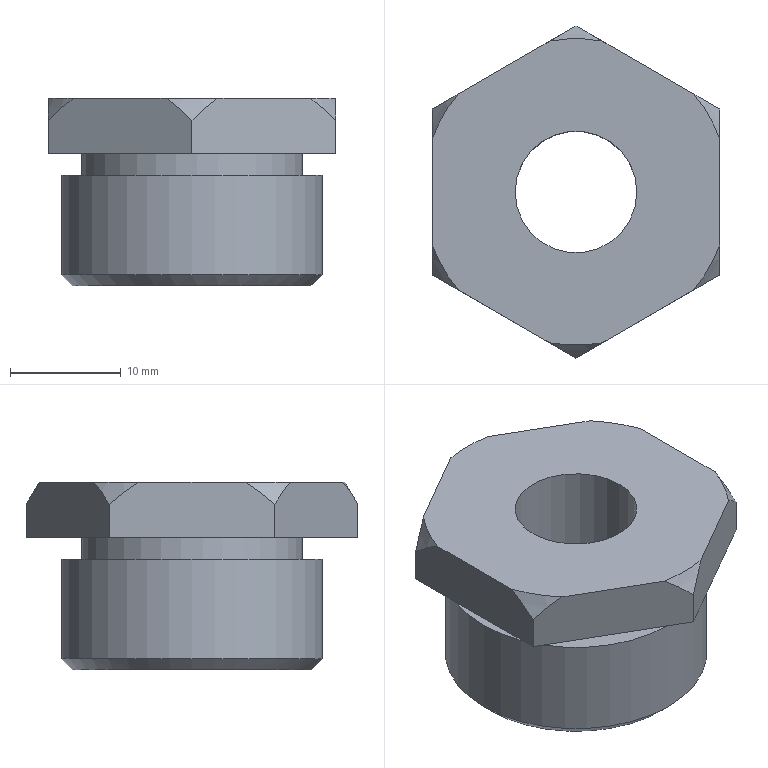Part | NX | features CYLINDER 3, CHAMFER 2, DATUM_CSYS 2, EXTRUDE 2, INTERSECT 1, SKETCH 1, SYMBOLIC_THREAD 1 | 1 solid | 20 faces | volume 6271 mm3 | plane 10 | cone 7 | cylinder 3 | commonest cylinder face diameters 11 x1 20 x1 23.607 x1